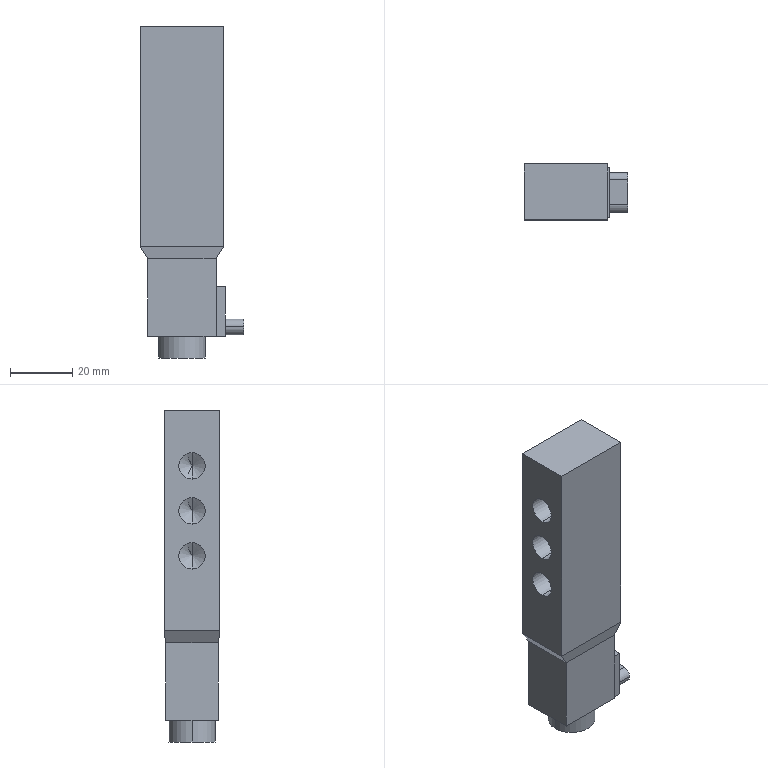Part | STEP file | single solenoid valve MVSD-180-4E1 | 1 solid | 47 faces | box 33.5 x 18 x 107 mm | volume 44857 mm3 | plane 22 | cylinder 15 | cone 10 | commonest cylinder face diameters 8.5 x10 5 x3 15 x2